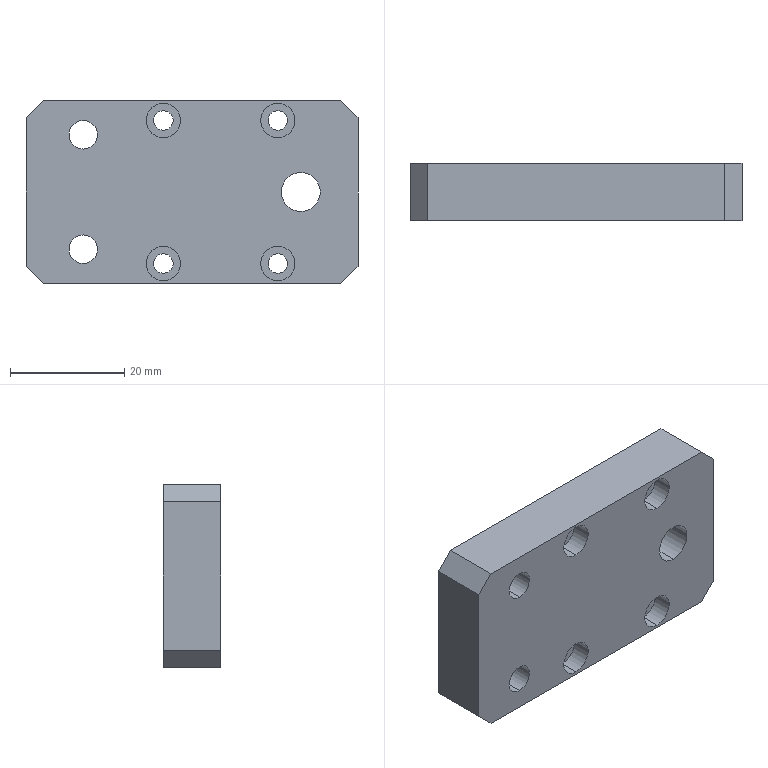Part | SolidWorks | features HoleWzd 3, Chamfer 1, Extrusion 1 | 1 solid | 36 faces | box 58 x 10 x 32 mm | volume 17000 mm3 | cylinder 22 | plane 14 | commonest cylinder face diameters 3.4 x8 6 x8 5 x4 6.8 x2
STEP:
#1=CARTESIAN_POINT('',(19.,10.,-3.4));
#2=VERTEX_POINT('',#1);
#3=CARTESIAN_POINT('',(19.,10.,3.4));
#4=VERTEX_POINT('',#3);
#5=CARTESIAN_POINT('',(19.,10.,0.));
#6=DIRECTION('',(0.,1.,0.));
#7=DIRECTION('',(0.,0.,1.));
#8=AXIS2_PLACEMENT_3D('',#5,#6,#7);
#9=CIRCLE('',#8,3.4);
#10=EDGE_CURVE('',#2,#4,#9,.T.);
#11=ORIENTED_EDGE('',*,*,#10,.T.);
#12=CARTESIAN_POINT('',(19.,0.,3.4));
#13=VERTEX_POINT('',#12);
#14=CARTESIAN_POINT('',(19.,0.,3.4));
#15=DIRECTION('',(0.,-1.,0.));
#16=VECTOR('',#15,1000.);
#17=LINE('',#14,#16);
#18=EDGE_CURVE('',#4,#13,#17,.T.);
#19=ORIENTED_EDGE('',*,*,#18,.T.);
#20=CARTESIAN_POINT('',(19.,0.,-3.4));
#21=VERTEX_POINT('',#20);
#22=CARTESIAN_POINT('',(19.,0.,0.));
#23=DIRECTION('',(0.,-1.,0.));
#24=DIRECTION('',(0.,0.,-1.));
#25=AXIS2_PLACEMENT_3D('',#22,#23,#24);
#26=CIRCLE('',#25,3.4);
#27=EDGE_CURVE('',#13,#21,#26,.T.);
#28=ORIENTED_EDGE('',*,*,#27,.T.);
#29=CARTESIAN_POINT('',(19.,0.,-3.4));
#30=DIRECTION('',(0.,-1.,0.));
#31=VECTOR('',#30,1000.);
#32=LINE('',#29,#31);
#33=EDGE_CURVE('',#2,#21,#32,.T.);
#34=ORIENTED_EDGE('',*,*,#33,.F.);
#35=EDGE_LOOP('',(#11,#19,#28,#34));
#36=FACE_OUTER_BOUND('',#35,.T.);
#37=CARTESIAN_POINT('',(19.,0.,0.));
#38=DIRECTION('',(0.,-1.,0.));
#39=DIRECTION('',(0.,0.,-1.));
#40=AXIS2_PLACEMENT_3D('',#37,#38,#39);
#41=CYLINDRICAL_SURFACE('',#40,3.4);
#42=ADVANCED_FACE('',(#36),#41,.F.);
#43=CARTESIAN_POINT('',(-19.,10.,-12.5));
#44=VERTEX_POINT('',#43);
#45=CARTESIAN_POINT('',(-19.,10.,-7.5));
#46=VERTEX_POINT('',#45);
#47=CARTESIAN_POINT('',(-19.,10.,-10.));
#48=DIRECTION('',(0.,1.,0.));
#49=DIRECTION('',(0.,0.,1.));
#50=AXIS2_PLACEMENT_3D('',#47,#48,#49);
#51=CIRCLE('',#50,2.5);
#52=EDGE_CURVE('',#44,#46,#51,.T.);
#53=ORIENTED_EDGE('',*,*,#52,.T.);
#54=CARTESIAN_POINT('',(-19.,0.,-7.5));
#55=VERTEX_POINT('',#54);
#56=CARTESIAN_POINT('',(-19.,0.,-7.5));
#57=DIRECTION('',(0.,-1.,0.));
#58=VECTOR('',#57,1000.);
#59=LINE('',#56,#58);
#60=EDGE_CURVE('',#46,#55,#59,.T.);
#61=ORIENTED_EDGE('',*,*,#60,.T.);
#62=CARTESIAN_POINT('',(-19.,0.,-12.5));
#63=VERTEX_POINT('',#62);
#64=CARTESIAN_POINT('',(-19.,0.,-10.));
#65=DIRECTION('',(0.,-1.,0.));
#66=DIRECTION('',(0.,0.,-1.));
#67=AXIS2_PLACEMENT_3D('',#64,#65,#66);
#68=CIRCLE('',#67,2.5);
#69=EDGE_CURVE('',#55,#63,#68,.T.);
#70=ORIENTED_EDGE('',*,*,#69,.T.);
#71=CARTESIAN_POINT('',(-19.,0.,-12.5));
#72=DIRECTION('',(0.,-1.,0.));
#73=VECTOR('',#72,1000.);
#74=LINE('',#71,#73);
#75=EDGE_CURVE('',#44,#63,#74,.T.);
#76=ORIENTED_EDGE('',*,*,#75,.F.);
#77=EDGE_LOOP('',(#53,#61,#70,#76));
#78=FACE_OUTER_BOUND('',#77,.T.);
#79=CARTESIAN_POINT('',(-19.,0.,-10.));
#80=DIRECTION('',(0.,-1.,0.));
#81=DIRECTION('',(0.,0.,-1.));
#82=AXIS2_PLACEMENT_3D('',#79,#80,#81);
#83=CYLINDRICAL_SURFACE('',#82,2.5);
#84=ADVANCED_FACE('',(#78),#83,.F.);
#85=CARTESIAN_POINT('',(-19.,10.,7.5));
#86=VERTEX_POINT('',#85);
#87=CARTESIAN_POINT('',(-19.,10.,12.5));
#88=VERTEX_POINT('',#87);
#89=CARTESIAN_POINT('',(-19.,10.,10.));
#90=DIRECTION('',(0.,1.,0.));
#91=DIRECTION('',(0.,0.,1.));
#92=AXIS2_PLACEMENT_3D('',#89,#90,#91);
#93=CIRCLE('',#92,2.5);
#94=EDGE_CURVE('',#86,#88,#93,.T.);
#95=ORIENTED_EDGE('',*,*,#94,.T.);
#96=CARTESIAN_POINT('',(-19.,0.,12.5));
#97=VERTEX_POINT('',#96);
#98=CARTESIAN_POINT('',(-19.,0.,12.5));
#99=DIRECTION('',(0.,-1.,0.));
#100=VECTOR('',#99,1000.);
#101=LINE('',#98,#100);
#102=EDGE_CURVE('',#88,#97,#101,.T.);
#103=ORIENTED_EDGE('',*,*,#102,.T.);
#104=CARTESIAN_POINT('',(-19.,0.,7.5));
#105=VERTEX_POINT('',#104);
#106=CARTESIAN_POINT('',(-19.,0.,10.));
#107=DIRECTION('',(0.,-1.,0.));
#108=DIRECTION('',(0.,0.,-1.));
#109=AXIS2_PLACEMENT_3D('',#106,#107,#108);
#110=CIRCLE('',#109,2.5);
#111=EDGE_CURVE('',#97,#105,#110,.T.);
#112=ORIENTED_EDGE('',*,*,#111,.T.);
#113=CARTESIAN_POINT('',(-19.,0.,7.5));
#114=DIRECTION('',(0.,-1.,0.));
#115=VECTOR('',#114,1000.);
#116=LINE('',#113,#115);
#117=EDGE_CURVE('',#86,#105,#116,.T.);
#118=ORIENTED_EDGE('',*,*,#117,.F.);
#119=EDGE_LOOP('',(#95,#103,#112,#118));
#120=FACE_OUTER_BOUND('',#119,.T.);
#121=CARTESIAN_POINT('',(-19.,0.,10.));
#122=DIRECTION('',(0.,-1.,0.));
#123=DIRECTION('',(0.,0.,-1.));
#124=AXIS2_PLACEMENT_3D('',#121,#122,#123);
#125=CYLINDRICAL_SURFACE('',#124,2.5);
#126=ADVANCED_FACE('',(#120),#125,.F.);
#127=CARTESIAN_POINT('',(15.,3.4,-9.5));
#128=VERTEX_POINT('',#127);
#129=CARTESIAN_POINT('',(15.,3.4,-15.5));
#130=VERTEX_POINT('',#129);
#131=CARTESIAN_POINT('',(15.,3.4,-12.5));
#132=DIRECTION('',(0.,-1.,0.));
#133=DIRECTION('',(0.,0.,-1.));
#134=AXIS2_PLACEMENT_3D('',#131,#132,#133);
#135=CIRCLE('',#134,3.);
#136=EDGE_CURVE('',#128,#130,#135,.T.);
#137=ORIENTED_EDGE('',*,*,#136,.F.);
#138=CARTESIAN_POINT('',(15.,0.,-9.5));
#139=VERTEX_POINT('',#138);
#140=CARTESIAN_POINT('',(15.,0.,-9.5));
#141=DIRECTION('',(0.,-1.,0.));
#142=VECTOR('',#141,1000.);
#143=LINE('',#140,#142);
#144=EDGE_CURVE('',#128,#139,#143,.T.);
#145=ORIENTED_EDGE('',*,*,#144,.T.);
#146=CARTESIAN_POINT('',(15.,0.,-15.5));
#147=VERTEX_POINT('',#146);
#148=CARTESIAN_POINT('',(15.,0.,-12.5));
#149=DIRECTION('',(0.,-1.,0.));
#150=DIRECTION('',(0.,0.,-1.));
#151=AXIS2_PLACEMENT_3D('',#148,#149,#150);
#152=CIRCLE('',#151,3.);
#153=EDGE_CURVE('',#139,#147,#152,.T.);
#154=ORIENTED_EDGE('',*,*,#153,.T.);
#155=CARTESIAN_POINT('',(15.,0.,-15.5));
#156=DIRECTION('',(0.,-1.,0.));
#157=VECTOR('',#156,1000.);
#158=LINE('',#155,#157);
#159=EDGE_CURVE('',#130,#147,#158,.T.);
#160=ORIENTED_EDGE('',*,*,#159,.F.);
#161=EDGE_LOOP('',(#137,#145,#154,#160));
#162=FACE_OUTER_BOUND('',#161,.T.);
#163=CARTESIAN_POINT('',(15.,0.,-12.5));
#164=DIRECTION('',(0.,-1.,0.));
#165=DIRECTION('',(0.,0.,-1.));
#166=AXIS2_PLACEMENT_3D('',#163,#164,#165);
#167=CYLINDRICAL_SURFACE('',#166,3.);
#168=ADVANCED_FACE('',(#162),#167,.F.);
#169=CARTESIAN_POINT('',(15.,10.,-14.2));
#170=VERTEX_POINT('',#169);
#171=CARTESIAN_POINT('',(15.,10.,-10.8));
#172=VERTEX_POINT('',#171);
#173=CARTESIAN_POINT('',(15.,10.,-12.5));
#174=DIRECTION('',(0.,1.,0.));
#175=DIRECTION('',(0.,0.,1.));
#176=AXIS2_PLACEMENT_3D('',#173,#174,#175);
#177=CIRCLE('',#176,1.7);
#178=EDGE_CURVE('',#170,#172,#177,.T.);
#179=ORIENTED_EDGE('',*,*,#178,.T.);
#180=CARTESIAN_POINT('',(15.,3.4,-10.8));
#181=VERTEX_POINT('',#180);
#182=CARTESIAN_POINT('',(15.,0.,-10.8));
#183=DIRECTION('',(0.,-1.,0.));
#184=VECTOR('',#183,1000.);
#185=LINE('',#182,#184);
#186=EDGE_CURVE('',#172,#181,#185,.T.);
#187=ORIENTED_EDGE('',*,*,#186,.T.);
#188=CARTESIAN_POINT('',(15.,3.4,-14.2));
#189=VERTEX_POINT('',#188);
#190=CARTESIAN_POINT('',(15.,3.4,-12.5));
#191=DIRECTION('',(0.,-1.,0.));
#192=DIRECTION('',(0.,0.,-1.));
#193=AXIS2_PLACEMENT_3D('',#190,#191,#192);
#194=CIRCLE('',#193,1.7);
#195=EDGE_CURVE('',#181,#189,#194,.T.);
#196=ORIENTED_EDGE('',*,*,#195,.T.);
#197=CARTESIAN_POINT('',(15.,0.,-14.2));
#198=DIRECTION('',(0.,-1.,0.));
#199=VECTOR('',#198,1000.);
#200=LINE('',#197,#199);
#201=EDGE_CURVE('',#170,#189,#200,.T.);
#202=ORIENTED_EDGE('',*,*,#201,.F.);
#203=EDGE_LOOP('',(#179,#187,#196,#202));
#204=FACE_OUTER_BOUND('',#203,.T.);
#205=CARTESIAN_POINT('',(15.,0.,-12.5));
#206=DIRECTION('',(0.,-1.,0.));
#207=DIRECTION('',(0.,0.,-1.));
#208=AXIS2_PLACEMENT_3D('',#205,#206,#207);
#209=CYLINDRICAL_SURFACE('',#208,1.7);
#210=ADVANCED_FACE('',(#204),#209,.F.);
#211=CARTESIAN_POINT('',(-5.,3.4,-9.5));
#212=VERTEX_POINT('',#211);
#213=CARTESIAN_POINT('',(-5.,3.4,-15.5));
#214=VERTEX_POINT('',#213);
#215=CARTESIAN_POINT('',(-5.,3.4,-12.5));
#216=DIRECTION('',(0.,-1.,0.));
#217=DIRECTION('',(0.,0.,-1.));
#218=AXIS2_PLACEMENT_3D('',#215,#216,#217);
#219=CIRCLE('',#218,3.);
#220=EDGE_CURVE('',#212,#214,#219,.T.);
#221=ORIENTED_EDGE('',*,*,#220,.F.);
#222=CARTESIAN_POINT('',(-5.,0.,-9.5));
#223=VERTEX_POINT('',#222);
#224=CARTESIAN_POINT('',(-5.,0.,-9.5));
#225=DIRECTION('',(0.,-1.,0.));
#226=VECTOR('',#225,1000.);
#227=LINE('',#224,#226);
#228=EDGE_CURVE('',#212,#223,#227,.T.);
#229=ORIENTED_EDGE('',*,*,#228,.T.);
#230=CARTESIAN_POINT('',(-5.,0.,-15.5));
#231=VERTEX_POINT('',#230);
#232=CARTESIAN_POINT('',(-5.,0.,-12.5));
#233=DIRECTION('',(0.,-1.,0.));
#234=DIRECTION('',(0.,0.,-1.));
#235=AXIS2_PLACEMENT_3D('',#232,#233,#234);
#236=CIRCLE('',#235,3.);
#237=EDGE_CURVE('',#223,#231,#236,.T.);
#238=ORIENTED_EDGE('',*,*,#237,.T.);
#239=CARTESIAN_POINT('',(-5.,0.,-15.5));
#240=DIRECTION('',(0.,-1.,0.));
#241=VECTOR('',#240,1000.);
#242=LINE('',#239,#241);
#243=EDGE_CURVE('',#214,#231,#242,.T.);
#244=ORIENTED_EDGE('',*,*,#243,.F.);
#245=EDGE_LOOP('',(#221,#229,#238,#244));
#246=FACE_OUTER_BOUND('',#245,.T.);
#247=CARTESIAN_POINT('',(-5.,0.,-12.5));
#248=DIRECTION('',(0.,-1.,0.));
#249=DIRECTION('',(0.,0.,-1.));
#250=AXIS2_PLACEMENT_3D('',#247,#248,#249);
#251=CYLINDRICAL_SURFACE('',#250,3.);
#252=ADVANCED_FACE('',(#246),#251,.F.);
#253=CARTESIAN_POINT('',(-5.,10.,-14.2));
#254=VERTEX_POINT('',#253);
#255=CARTESIAN_POINT('',(-5.,10.,-10.8));
#256=VERTEX_POINT('',#255);
#257=CARTESIAN_POINT('',(-5.,10.,-12.5));
#258=DIRECTION('',(0.,1.,0.));
#259=DIRECTION('',(0.,0.,1.));
#260=AXIS2_PLACEMENT_3D('',#257,#258,#259);
#261=CIRCLE('',#260,1.7);
#262=EDGE_CURVE('',#254,#256,#261,.T.);
#263=ORIENTED_EDGE('',*,*,#262,.T.);
#264=CARTESIAN_POINT('',(-5.,3.4,-10.8));
#265=VERTEX_POINT('',#264);
#266=CARTESIAN_POINT('',(-5.,0.,-10.8));
#267=DIRECTION('',(0.,-1.,0.));
#268=VECTOR('',#267,1000.);
#269=LINE('',#266,#268);
#270=EDGE_CURVE('',#256,#265,#269,.T.);
#271=ORIENTED_EDGE('',*,*,#270,.T.);
#272=CARTESIAN_POINT('',(-5.,3.4,-14.2));
#273=VERTEX_POINT('',#272);
#274=CARTESIAN_POINT('',(-5.,3.4,-12.5));
#275=DIRECTION('',(0.,-1.,0.));
#276=DIRECTION('',(0.,0.,-1.));
#277=AXIS2_PLACEMENT_3D('',#274,#275,#276);
#278=CIRCLE('',#277,1.7);
#279=EDGE_CURVE('',#265,#273,#278,.T.);
#280=ORIENTED_EDGE('',*,*,#279,.T.);
#281=CARTESIAN_POINT('',(-5.,0.,-14.2));
#282=DIRECTION('',(0.,-1.,0.));
#283=VECTOR('',#282,1000.);
#284=LINE('',#281,#283);
#285=EDGE_CURVE('',#254,#273,#284,.T.);
#286=ORIENTED_EDGE('',*,*,#285,.F.);
#287=EDGE_LOOP('',(#263,#271,#280,#286));
#288=FACE_OUTER_BOUND('',#287,.T.);
#289=CARTESIAN_POINT('',(-5.,0.,-12.5));
#290=DIRECTION('',(0.,-1.,0.));
#291=DIRECTION('',(0.,0.,-1.));
#292=AXIS2_PLACEMENT_3D('',#289,#290,#291);
#293=CYLINDRICAL_SURFACE('',#292,1.7);
#294=ADVANCED_FACE('',(#288),#293,.F.);
#295=CARTESIAN_POINT('',(15.,3.4,15.5));
#296=VERTEX_POINT('',#295);
#297=CARTESIAN_POINT('',(15.,3.4,9.5));
#298=VERTEX_POINT('',#297);
#299=CARTESIAN_POINT('',(15.,3.4,12.5));
#300=DIRECTION('',(0.,-1.,0.));
#301=DIRECTION('',(0.,0.,-1.));
#302=AXIS2_PLACEMENT_3D('',#299,#300,#301);
#303=CIRCLE('',#302,3.);
#304=EDGE_CURVE('',#296,#298,#303,.T.);
#305=ORIENTED_EDGE('',*,*,#304,.F.);
#306=CARTESIAN_POINT('',(15.,0.,15.5));
#307=VERTEX_POINT('',#306);
#308=CARTESIAN_POINT('',(15.,0.,15.5));
#309=DIRECTION('',(0.,-1.,0.));
#310=VECTOR('',#309,1000.);
#311=LINE('',#308,#310);
#312=EDGE_CURVE('',#296,#307,#311,.T.);
#313=ORIENTED_EDGE('',*,*,#312,.T.);
#314=CARTESIAN_POINT('',(15.,0.,9.5));
#315=VERTEX_POINT('',#314);
#316=CARTESIAN_POINT('',(15.,0.,12.5));
#317=DIRECTION('',(0.,-1.,0.));
#318=DIRECTION('',(0.,0.,-1.));
#319=AXIS2_PLACEMENT_3D('',#316,#317,#318);
#320=CIRCLE('',#319,3.);
#321=EDGE_CURVE('',#307,#315,#320,.T.);
#322=ORIENTED_EDGE('',*,*,#321,.T.);
#323=CARTESIAN_POINT('',(15.,0.,9.5));
#324=DIRECTION('',(0.,-1.,0.));
#325=VECTOR('',#324,1000.);
#326=LINE('',#323,#325);
#327=EDGE_CURVE('',#298,#315,#326,.T.);
#328=ORIENTED_EDGE('',*,*,#327,.F.);
#329=EDGE_LOOP('',(#305,#313,#322,#328));
#330=FACE_OUTER_BOUND('',#329,.T.);
#331=CARTESIAN_POINT('',(15.,0.,12.5));
#332=DIRECTION('',(0.,-1.,0.));
#333=DIRECTION('',(0.,0.,-1.));
#334=AXIS2_PLACEMENT_3D('',#331,#332,#333);
#335=CYLINDRICAL_SURFACE('',#334,3.);
#336=ADVANCED_FACE('',(#330),#335,.F.);
#337=CARTESIAN_POINT('',(15.,10.,10.8));
#338=VERTEX_POINT('',#337);
#339=CARTESIAN_POINT('',(15.,10.,14.2));
#340=VERTEX_POINT('',#339);
#341=CARTESIAN_POINT('',(15.,10.,12.5));
#342=DIRECTION('',(0.,1.,0.));
#343=DIRECTION('',(0.,0.,1.));
#344=AXIS2_PLACEMENT_3D('',#341,#342,#343);
#345=CIRCLE('',#344,1.7);
#346=EDGE_CURVE('',#338,#340,#345,.T.);
#347=ORIENTED_EDGE('',*,*,#346,.T.);
#348=CARTESIAN_POINT('',(15.,3.4,14.2));
#349=VERTEX_POINT('',#348);
#350=CARTESIAN_POINT('',(15.,0.,14.2));
#351=DIRECTION('',(0.,-1.,0.));
#352=VECTOR('',#351,1000.);
#353=LINE('',#350,#352);
#354=EDGE_CURVE('',#340,#349,#353,.T.);
#355=ORIENTED_EDGE('',*,*,#354,.T.);
#356=CARTESIAN_POINT('',(15.,3.4,10.8));
#357=VERTEX_POINT('',#356);
#358=CARTESIAN_POINT('',(15.,3.4,12.5));
#359=DIRECTION('',(0.,-1.,0.));
#360=DIRECTION('',(0.,0.,-1.));
#361=AXIS2_PLACEMENT_3D('',#358,#359,#360);
#362=CIRCLE('',#361,1.7);
#363=EDGE_CURVE('',#349,#357,#362,.T.);
#364=ORIENTED_EDGE('',*,*,#363,.T.);
#365=CARTESIAN_POINT('',(15.,0.,10.8));
#366=DIRECTION('',(0.,-1.,0.));
#367=VECTOR('',#366,1000.);
#368=LINE('',#365,#367);
#369=EDGE_CURVE('',#338,#357,#368,.T.);
#370=ORIENTED_EDGE('',*,*,#369,.F.);
#371=EDGE_LOOP('',(#347,#355,#364,#370));
#372=FACE_OUTER_BOUND('',#371,.T.);
#373=CARTESIAN_POINT('',(15.,0.,12.5));
#374=DIRECTION('',(0.,-1.,0.));
#375=DIRECTION('',(0.,0.,-1.));
#376=AXIS2_PLACEMENT_3D('',#373,#374,#375);
#377=CYLINDRICAL_SURFACE('',#376,1.7);
#378=ADVANCED_FACE('',(#372),#377,.F.);
#379=CARTESIAN_POINT('',(-5.,3.4,15.5));
#380=VERTEX_POINT('',#379);
#381=CARTESIAN_POINT('',(-5.,3.4,9.5));
#382=VERTEX_POINT('',#381);
#383=CARTESIAN_POINT('',(-5.,3.4,12.5));
#384=DIRECTION('',(0.,-1.,0.));
#385=DIRECTION('',(0.,0.,-1.));
#386=AXIS2_PLACEMENT_3D('',#383,#384,#385);
#387=CIRCLE('',#386,3.);
#388=EDGE_CURVE('',#380,#382,#387,.T.);
#389=ORIENTED_EDGE('',*,*,#388,.F.);
#390=CARTESIAN_POINT('',(-5.,0.,15.5));
#391=VERTEX_POINT('',#390);
#392=CARTESIAN_POINT('',(-5.,0.,15.5));
#393=DIRECTION('',(0.,-1.,0.));
#394=VECTOR('',#393,1000.);
#395=LINE('',#392,#394);
#396=EDGE_CURVE('',#380,#391,#395,.T.);
#397=ORIENTED_EDGE('',*,*,#396,.T.);
#398=CARTESIAN_POINT('',(-5.,0.,9.5));
#399=VERTEX_POINT('',#398);
#400=CARTESIAN_POINT('',(-5.,0.,12.5));
#401=DIRECTION('',(0.,-1.,0.));
#402=DIRECTION('',(0.,0.,-1.));
#403=AXIS2_PLACEMENT_3D('',#400,#401,#402);
#404=CIRCLE('',#403,3.);
#405=EDGE_CURVE('',#391,#399,#404,.T.);
#406=ORIENTED_EDGE('',*,*,#405,.T.);
#407=CARTESIAN_POINT('',(-5.,0.,9.5));
#408=DIRECTION('',(0.,-1.,0.));
#409=VECTOR('',#408,1000.);
#410=LINE('',#407,#409);
#411=EDGE_CURVE('',#382,#399,#410,.T.);
#412=ORIENTED_EDGE('',*,*,#411,.F.);
#413=EDGE_LOOP('',(#389,#397,#406,#412));
#414=FACE_OUTER_BOUND('',#413,.T.);
#415=CARTESIAN_POINT('',(-5.,0.,12.5));
#416=DIRECTION('',(0.,-1.,0.));
#417=DIRECTION('',(0.,0.,-1.));
#418=AXIS2_PLACEMENT_3D('',#415,#416,#417);
#419=CYLINDRICAL_SURFACE('',#418,3.);
#420=ADVANCED_FACE('',(#414),#419,.F.);
#421=CARTESIAN_POINT('',(-5.,10.,10.8));
#422=VERTEX_POINT('',#421);
#423=CARTESIAN_POINT('',(-5.,10.,14.2));
#424=VERTEX_POINT('',#423);
#425=CARTESIAN_POINT('',(-5.,10.,12.5));
#426=DIRECTION('',(0.,1.,0.));
#427=DIRECTION('',(0.,0.,1.));
#428=AXIS2_PLACEMENT_3D('',#425,#426,#427);
#429=CIRCLE('',#428,1.7);
#430=EDGE_CURVE('',#422,#424,#429,.T.);
#431=ORIENTED_EDGE('',*,*,#430,.T.);
#432=CARTESIAN_POINT('',(-5.,3.4,14.2));
#433=VERTEX_POINT('',#432);
#434=CARTESIAN_POINT('',(-5.,0.,14.2));
#435=DIRECTION('',(0.,-1.,0.));
#436=VECTOR('',#435,1000.);
#437=LINE('',#434,#436);
#438=EDGE_CURVE('',#424,#433,#437,.T.);
#439=ORIENTED_EDGE('',*,*,#438,.T.);
#440=CARTESIAN_POINT('',(-5.,3.4,10.8));
#441=VERTEX_POINT('',#440);
#442=CARTESIAN_POINT('',(-5.,3.4,12.5));
#443=DIRECTION('',(0.,-1.,0.));
#444=DIRECTION('',(0.,0.,-1.));
#445=AXIS2_PLACEMENT_3D('',#442,#443,#444);
#446=CIRCLE('',#445,1.7);
#447=EDGE_CURVE('',#433,#441,#446,.T.);
#448=ORIENTED_EDGE('',*,*,#447,.T.);
#449=CARTESIAN_POINT('',(-5.,0.,10.8));
#450=DIRECTION('',(0.,-1.,0.));
#451=VECTOR('',#450,1000.);
#452=LINE('',#449,#451);
#453=EDGE_CURVE('',#422,#441,#452,.T.);
#454=ORIENTED_EDGE('',*,*,#453,.F.);
#455=EDGE_LOOP('',(#431,#439,#448,#454));
#456=FACE_OUTER_BOUND('',#455,.T.);
#457=CARTESIAN_POINT('',(-5.,0.,12.5));
#458=DIRECTION('',(0.,-1.,0.));
#459=DIRECTION('',(0.,0.,-1.));
#460=AXIS2_PLACEMENT_3D('',#457,#458,#459);
#461=CYLINDRICAL_SURFACE('',#460,1.7);
#462=ADVANCED_FACE('',(#456),#461,.F.);
#463=CARTESIAN_POINT('',(29.,0.,13.));
#464=VERTEX_POINT('',#463);
#465=CARTESIAN_POINT('',(29.,0.,-13.));
#466=VERTEX_POINT('',#465);
#467=CARTESIAN_POINT('',(29.,0.,-16.));
#468=DIRECTION('',(0.,0.,-1.));
#469=VECTOR('',#468,1000.);
#470=LINE('',#467,#469);
#471=EDGE_CURVE('',#464,#466,#470,.T.);
#472=ORIENTED_EDGE('',*,*,#471,.T.);
#473=CARTESIAN_POINT('',(29.,10.,-13.));
#474=VERTEX_POINT('',#473);
#475=CARTESIAN_POINT('',(29.,10.,-13.));
#476=DIRECTION('',(0.,1.,0.));
#477=VECTOR('',#476,1000.);
#478=LINE('',#475,#477);
#479=EDGE_CURVE('',#466,#474,#478,.T.);
#480=ORIENTED_EDGE('',*,*,#479,.T.);
#481=CARTESIAN_POINT('',(29.,10.,13.));
#482=VERTEX_POINT('',#481);
#483=CARTESIAN_POINT('',(29.,10.,-16.));
#484=DIRECTION('',(0.,0.,-1.));
#485=VECTOR('',#484,1000.);
#486=LINE('',#483,#485);
#487=EDGE_CURVE('',#482,#474,#486,.T.);
#488=ORIENTED_EDGE('',*,*,#487,.F.);
#489=CARTESIAN_POINT('',(29.,10.,13.));
#490=DIRECTION('',(0.,-1.,0.));
#491=VECTOR('',#490,1000.);
#492=LINE('',#489,#491);
#493=EDGE_CURVE('',#482,#464,#492,.T.);
#494=ORIENTED_EDGE('',*,*,#493,.T.);
#495=EDGE_LOOP('',(#472,#480,#488,#494));
#496=FACE_OUTER_BOUND('',#495,.T.);
#497=CARTESIAN_POINT('',(29.,10.,-16.));
#498=DIRECTION('',(-1.,0.,0.));
#499=DIRECTION('',(0.,0.,1.));
#500=AXIS2_PLACEMENT_3D('',#497,#498,#499);
#501=PLANE('',#500);
#502=ADVANCED_FACE('',(#496),#501,.F.);
#503=CARTESIAN_POINT('',(26.,0.,-16.));
#504=VERTEX_POINT('',#503);
#505=CARTESIAN_POINT('',(-26.,0.,-16.));
#506=VERTEX_POINT('',#505);
#507=CARTESIAN_POINT('',(-29.,0.,-16.));
#508=DIRECTION('',(-1.,0.,0.));
#509=VECTOR('',#508,1000.);
#510=LINE('',#507,#509);
#511=EDGE_CURVE('',#504,#506,#510,.T.);
#512=ORIENTED_EDGE('',*,*,#511,.T.);
#513=CARTESIAN_POINT('',(-26.,10.,-16.));
#514=VERTEX_POINT('',#513);
#515=CARTESIAN_POINT('',(-26.,10.,-16.));
#516=DIRECTION('',(0.,1.,0.));
#517=VECTOR('',#516,1000.);
#518=LINE('',#515,#517);
#519=EDGE_CURVE('',#506,#514,#518,.T.);
#520=ORIENTED_EDGE('',*,*,#519,.T.);
#521=CARTESIAN_POINT('',(26.,10.,-16.));
#522=VERTEX_POINT('',#521);
#523=CARTESIAN_POINT('',(-29.,10.,-16.));
#524=DIRECTION('',(-1.,0.,0.));
#525=VECTOR('',#524,1000.);
#526=LINE('',#523,#525);
#527=EDGE_CURVE('',#522,#514,#526,.T.);
#528=ORIENTED_EDGE('',*,*,#527,.F.);
#529=CARTESIAN_POINT('',(26.,10.,-16.));
#530=DIRECTION('',(0.,-1.,0.));
#531=VECTOR('',#530,1000.);
#532=LINE('',#529,#531);
#533=EDGE_CURVE('',#522,#504,#532,.T.);
#534=ORIENTED_EDGE('',*,*,#533,.T.);
#535=EDGE_LOOP('',(#512,#520,#528,#534));
#536=FACE_OUTER_BOUND('',#535,.T.);
#537=CARTESIAN_POINT('',(-29.,10.,-16.));
#538=DIRECTION('',(0.,0.,1.));
#539=DIRECTION('',(1.,0.,0.));
#540=AXIS2_PLACEMENT_3D('',#537,#538,#539);
#541=PLANE('',#540);
#542=ADVANCED_FACE('',(#536),#541,.F.);
#543=CARTESIAN_POINT('',(-29.,10.,-13.));
#544=VERTEX_POINT('',#543);
#545=CARTESIAN_POINT('',(-29.,10.,13.));
#546=VERTEX_POINT('',#545);
#547=CARTESIAN_POINT('',(-29.,10.,-16.));
#548=DIRECTION('',(0.,0.,1.));
#549=VECTOR('',#548,1000.);
#550=LINE('',#547,#549);
#551=EDGE_CURVE('',#544,#546,#550,.T.);
#552=ORIENTED_EDGE('',*,*,#551,.F.);
#553=CARTESIAN_POINT('',(-29.,0.,-13.));
#554=VERTEX_POINT('',#553);
#555=CARTESIAN_POINT('',(-29.,10.,-13.));
#556=DIRECTION('',(0.,-1.,0.));
#557=VECTOR('',#556,1000.);
#558=LINE('',#555,#557);
#559=EDGE_CURVE('',#544,#554,#558,.T.);
#560=ORIENTED_EDGE('',*,*,#559,.T.);
#561=CARTESIAN_POINT('',(-29.,0.,13.));
#562=VERTEX_POINT('',#561);
#563=CARTESIAN_POINT('',(-29.,0.,-16.));
#564=DIRECTION('',(0.,0.,1.));
#565=VECTOR('',#564,1000.);
#566=LINE('',#563,#565);
#567=EDGE_CURVE('',#554,#562,#566,.T.);
#568=ORIENTED_EDGE('',*,*,#567,.T.);
#569=CARTESIAN_POINT('',(-29.,10.,13.));
#570=DIRECTION('',(0.,1.,0.));
#571=VECTOR('',#570,1000.);
#572=LINE('',#569,#571);
#573=EDGE_CURVE('',#562,#546,#572,.T.);
#574=ORIENTED_EDGE('',*,*,#573,.T.);
#575=EDGE_LOOP('',(#552,#560,#568,#574));
#576=FACE_OUTER_BOUND('',#575,.T.);
#577=CARTESIAN_POINT('',(-29.,10.,-16.));
#578=DIRECTION('',(1.,0.,0.));
#579=DIRECTION('',(0.,0.,-1.));
#580=AXIS2_PLACEMENT_3D('',#577,#578,#579);
#581=PLANE('',#580);
#582=ADVANCED_FACE('',(#576),#581,.F.);
#583=CARTESIAN_POINT('',(-26.,10.,16.));
#584=VERTEX_POINT('',#583);
#585=CARTESIAN_POINT('',(26.,10.,16.));
#586=VERTEX_POINT('',#585);
#587=CARTESIAN_POINT('',(-29.,10.,16.));
#588=DIRECTION('',(1.,0.,0.));
#589=VECTOR('',#588,1000.);
#590=LINE('',#587,#589);
#591=EDGE_CURVE('',#584,#586,#590,.T.);
#592=ORIENTED_EDGE('',*,*,#591,.F.);
#593=CARTESIAN_POINT('',(-26.,0.,16.));
#594=VERTEX_POINT('',#593);
#595=CARTESIAN_POINT('',(-26.,10.,16.));
#596=DIRECTION('',(0.,-1.,0.));
#597=VECTOR('',#596,1000.);
#598=LINE('',#595,#597);
#599=EDGE_CURVE('',#584,#594,#598,.T.);
#600=ORIENTED_EDGE('',*,*,#599,.T.);
#601=CARTESIAN_POINT('',(26.,0.,16.));
#602=VERTEX_POINT('',#601);
#603=CARTESIAN_POINT('',(-29.,0.,16.));
#604=DIRECTION('',(1.,0.,0.));
#605=VECTOR('',#604,1000.);
#606=LINE('',#603,#605);
#607=EDGE_CURVE('',#594,#602,#606,.T.);
#608=ORIENTED_EDGE('',*,*,#607,.T.);
#609=CARTESIAN_POINT('',(26.,10.,16.));
#610=DIRECTION('',(0.,1.,0.));
#611=VECTOR('',#610,1000.);
#612=LINE('',#609,#611);
#613=EDGE_CURVE('',#602,#586,#612,.T.);
#614=ORIENTED_EDGE('',*,*,#613,.T.);
#615=EDGE_LOOP('',(#592,#600,#608,#614));
#616=FACE_OUTER_BOUND('',#615,.T.);
#617=CARTESIAN_POINT('',(-29.,10.,16.));
#618=DIRECTION('',(0.,0.,-1.));
#619=DIRECTION('',(-1.,0.,0.));
#620=AXIS2_PLACEMENT_3D('',#617,#618,#619);
#621=PLANE('',#620);
#622=ADVANCED_FACE('',(#616),#621,.F.);
#623=ORIENTED_EDGE('',*,*,#10,.F.);
#624=CARTESIAN_POINT('',(19.,10.,0.));
#625=DIRECTION('',(0.,1.,0.));
#626=DIRECTION('',(0.,0.,1.));
#627=AXIS2_PLACEMENT_3D('',#624,#625,#626);
#628=CIRCLE('',#627,3.4);
#629=EDGE_CURVE('',#4,#2,#628,.T.);
#630=ORIENTED_EDGE('',*,*,#629,.F.);
#631=EDGE_LOOP('',(#623,#630));
#632=FACE_BOUND('',#631,.T.);
#633=ORIENTED_EDGE('',*,*,#52,.F.);
#634=CARTESIAN_POINT('',(-19.,10.,-10.));
#635=DIRECTION('',(0.,1.,0.));
#636=DIRECTION('',(0.,0.,1.));
#637=AXIS2_PLACEMENT_3D('',#634,#635,#636);
#638=CIRCLE('',#637,2.5);
#639=EDGE_CURVE('',#46,#44,#638,.T.);
#640=ORIENTED_EDGE('',*,*,#639,.F.);
#641=EDGE_LOOP('',(#633,#640));
#642=FACE_BOUND('',#641,.T.);
#643=ORIENTED_EDGE('',*,*,#94,.F.);
#644=CARTESIAN_POINT('',(-19.,10.,10.));
#645=DIRECTION('',(0.,1.,0.));
#646=DIRECTION('',(0.,0.,1.));
#647=AXIS2_PLACEMENT_3D('',#644,#645,#646);
#648=CIRCLE('',#647,2.5);
#649=EDGE_CURVE('',#88,#86,#648,.T.);
#650=ORIENTED_EDGE('',*,*,#649,.F.);
#651=EDGE_LOOP('',(#643,#650));
#652=FACE_BOUND('',#651,.T.);
#653=ORIENTED_EDGE('',*,*,#178,.F.);
#654=CARTESIAN_POINT('',(15.,10.,-12.5));
#655=DIRECTION('',(0.,1.,0.));
#656=DIRECTION('',(0.,0.,1.));
#657=AXIS2_PLACEMENT_3D('',#654,#655,#656);
#658=CIRCLE('',#657,1.7);
#659=EDGE_CURVE('',#172,#170,#658,.T.);
#660=ORIENTED_EDGE('',*,*,#659,.F.);
#661=EDGE_LOOP('',(#653,#660));
#662=FACE_BOUND('',#661,.T.);
#663=ORIENTED_EDGE('',*,*,#262,.F.);
#664=CARTESIAN_POINT('',(-5.,10.,-12.5));
#665=DIRECTION('',(0.,1.,0.));
#666=DIRECTION('',(0.,0.,1.));
#667=AXIS2_PLACEMENT_3D('',#664,#665,#666);
#668=CIRCLE('',#667,1.7);
#669=EDGE_CURVE('',#256,#254,#668,.T.);
#670=ORIENTED_EDGE('',*,*,#669,.F.);
#671=EDGE_LOOP('',(#663,#670));
#672=FACE_BOUND('',#671,.T.);
#673=ORIENTED_EDGE('',*,*,#346,.F.);
#674=CARTESIAN_POINT('',(15.,10.,12.5));
#675=DIRECTION('',(0.,1.,0.));
#676=DIRECTION('',(0.,0.,1.));
#677=AXIS2_PLACEMENT_3D('',#674,#675,#676);
#678=CIRCLE('',#677,1.7);
#679=EDGE_CURVE('',#340,#338,#678,.T.);
#680=ORIENTED_EDGE('',*,*,#679,.F.);
#681=EDGE_LOOP('',(#673,#680));
#682=FACE_BOUND('',#681,.T.);
#683=ORIENTED_EDGE('',*,*,#430,.F.);
#684=CARTESIAN_POINT('',(-5.,10.,12.5));
#685=DIRECTION('',(0.,1.,0.));
#686=DIRECTION('',(0.,0.,1.));
#687=AXIS2_PLACEMENT_3D('',#684,#685,#686);
#688=CIRCLE('',#687,1.7);
#689=EDGE_CURVE('',#424,#422,#688,.T.);
#690=ORIENTED_EDGE('',*,*,#689,.F.);
#691=EDGE_LOOP('',(#683,#690));
#692=FACE_BOUND('',#691,.T.);
#693=ORIENTED_EDGE('',*,*,#527,.T.);
#694=CARTESIAN_POINT('',(-21.,10.,-21.));
#695=DIRECTION('',(-0.7071,0.,0.7071));
#696=VECTOR('',#695,1000.);
#697=LINE('',#694,#696);
#698=EDGE_CURVE('',#514,#544,#697,.T.);
#699=ORIENTED_EDGE('',*,*,#698,.T.);
#700=ORIENTED_EDGE('',*,*,#551,.T.);
#701=CARTESIAN_POINT('',(-21.,10.,21.));
#702=DIRECTION('',(0.7071,0.,0.7071));
#703=VECTOR('',#702,1000.);
#704=LINE('',#701,#703);
#705=EDGE_CURVE('',#546,#584,#704,.T.);
#706=ORIENTED_EDGE('',*,*,#705,.T.);
#707=ORIENTED_EDGE('',*,*,#591,.T.);
#708=CARTESIAN_POINT('',(21.,10.,21.));
#709=DIRECTION('',(0.7071,0.,-0.7071));
#710=VECTOR('',#709,1000.);
#711=LINE('',#708,#710);
#712=EDGE_CURVE('',#586,#482,#711,.T.);
#713=ORIENTED_EDGE('',*,*,#712,.T.);
#714=ORIENTED_EDGE('',*,*,#487,.T.);
#715=CARTESIAN_POINT('',(21.,10.,-21.));
#716=DIRECTION('',(-0.7071,0.,-0.7071));
#717=VECTOR('',#716,1000.);
#718=LINE('',#715,#717);
#719=EDGE_CURVE('',#474,#522,#718,.T.);
#720=ORIENTED_EDGE('',*,*,#719,.T.);
#721=EDGE_LOOP('',(#693,#699,#700,#706,#707,#713,#714,#720));
#722=FACE_OUTER_BOUND('',#721,.T.);
#723=CARTESIAN_POINT('',(0.,10.,0.));
#724=DIRECTION('',(0.,1.,0.));
#725=DIRECTION('',(0.,0.,1.));
#726=AXIS2_PLACEMENT_3D('',#723,#724,#725);
#727=PLANE('',#726);
#728=ADVANCED_FACE('',(#632,#642,#652,#662,#672,#682,#692,#722),#727,.T.);
#729=CARTESIAN_POINT('',(19.,0.,0.));
#730=DIRECTION('',(0.,-1.,0.));
#731=DIRECTION('',(0.,0.,-1.));
#732=AXIS2_PLACEMENT_3D('',#729,#730,#731);
#733=CIRCLE('',#732,3.4);
#734=EDGE_CURVE('',#21,#13,#733,.T.);
#735=ORIENTED_EDGE('',*,*,#734,.F.);
#736=ORIENTED_EDGE('',*,*,#27,.F.);
#737=EDGE_LOOP('',(#735,#736));
#738=FACE_BOUND('',#737,.T.);
#739=CARTESIAN_POINT('',(-19.,0.,-10.));
#740=DIRECTION('',(0.,-1.,0.));
#741=DIRECTION('',(0.,0.,-1.));
#742=AXIS2_PLACEMENT_3D('',#739,#740,#741);
#743=CIRCLE('',#742,2.5);
#744=EDGE_CURVE('',#63,#55,#743,.T.);
#745=ORIENTED_EDGE('',*,*,#744,.F.);
#746=ORIENTED_EDGE('',*,*,#69,.F.);
#747=EDGE_LOOP('',(#745,#746));
#748=FACE_BOUND('',#747,.T.);
#749=CARTESIAN_POINT('',(-19.,0.,10.));
#750=DIRECTION('',(0.,-1.,0.));
#751=DIRECTION('',(0.,0.,-1.));
#752=AXIS2_PLACEMENT_3D('',#749,#750,#751);
#753=CIRCLE('',#752,2.5);
#754=EDGE_CURVE('',#105,#97,#753,.T.);
#755=ORIENTED_EDGE('',*,*,#754,.F.);
#756=ORIENTED_EDGE('',*,*,#111,.F.);
#757=EDGE_LOOP('',(#755,#756));
#758=FACE_BOUND('',#757,.T.);
#759=CARTESIAN_POINT('',(15.,0.,-12.5));
#760=DIRECTION('',(0.,-1.,0.));
#761=DIRECTION('',(0.,0.,-1.));
#762=AXIS2_PLACEMENT_3D('',#759,#760,#761);
#763=CIRCLE('',#762,3.);
#764=EDGE_CURVE('',#147,#139,#763,.T.);
#765=ORIENTED_EDGE('',*,*,#764,.F.);
#766=ORIENTED_EDGE('',*,*,#153,.F.);
#767=EDGE_LOOP('',(#765,#766));
#768=FACE_BOUND('',#767,.T.);
#769=CARTESIAN_POINT('',(-5.,0.,-12.5));
#770=DIRECTION('',(0.,-1.,0.));
#771=DIRECTION('',(0.,0.,-1.));
#772=AXIS2_PLACEMENT_3D('',#769,#770,#771);
#773=CIRCLE('',#772,3.);
#774=EDGE_CURVE('',#231,#223,#773,.T.);
#775=ORIENTED_EDGE('',*,*,#774,.F.);
#776=ORIENTED_EDGE('',*,*,#237,.F.);
#777=EDGE_LOOP('',(#775,#776));
#778=FACE_BOUND('',#777,.T.);
#779=CARTESIAN_POINT('',(15.,0.,12.5));
#780=DIRECTION('',(0.,-1.,0.));
#781=DIRECTION('',(0.,0.,-1.));
#782=AXIS2_PLACEMENT_3D('',#779,#780,#781);
#783=CIRCLE('',#782,3.);
#784=EDGE_CURVE('',#315,#307,#783,.T.);
#785=ORIENTED_EDGE('',*,*,#784,.F.);
#786=ORIENTED_EDGE('',*,*,#321,.F.);
#787=EDGE_LOOP('',(#785,#786));
#788=FACE_BOUND('',#787,.T.);
#789=CARTESIAN_POINT('',(-5.,0.,12.5));
#790=DIRECTION('',(0.,-1.,0.));
#791=DIRECTION('',(0.,0.,-1.));
#792=AXIS2_PLACEMENT_3D('',#789,#790,#791);
#793=CIRCLE('',#792,3.);
#794=EDGE_CURVE('',#399,#391,#793,.T.);
#795=ORIENTED_EDGE('',*,*,#794,.F.);
#796=ORIENTED_EDGE('',*,*,#405,.F.);
#797=EDGE_LOOP('',(#795,#796));
#798=FACE_BOUND('',#797,.T.);
#799=ORIENTED_EDGE('',*,*,#567,.F.);
#800=CARTESIAN_POINT('',(-29.,0.,-13.));
#801=DIRECTION('',(0.7071,0.,-0.7071));
#802=VECTOR('',#801,1000.);
#803=LINE('',#800,#802);
#804=EDGE_CURVE('',#554,#506,#803,.T.);
#805=ORIENTED_EDGE('',*,*,#804,.T.);
#806=ORIENTED_EDGE('',*,*,#511,.F.);
#807=CARTESIAN_POINT('',(26.,0.,-16.));
#808=DIRECTION('',(0.7071,0.,0.7071));
#809=VECTOR('',#808,1000.);
#810=LINE('',#807,#809);
#811=EDGE_CURVE('',#504,#466,#810,.T.);
#812=ORIENTED_EDGE('',*,*,#811,.T.);
#813=ORIENTED_EDGE('',*,*,#471,.F.);
#814=CARTESIAN_POINT('',(29.,0.,13.));
#815=DIRECTION('',(-0.7071,0.,0.7071));
#816=VECTOR('',#815,1000.);
#817=LINE('',#814,#816);
#818=EDGE_CURVE('',#464,#602,#817,.T.);
#819=ORIENTED_EDGE('',*,*,#818,.T.);
#820=ORIENTED_EDGE('',*,*,#607,.F.);
#821=CARTESIAN_POINT('',(-26.,0.,16.));
#822=DIRECTION('',(-0.7071,0.,-0.7071));
#823=VECTOR('',#822,1000.);
#824=LINE('',#821,#823);
#825=EDGE_CURVE('',#594,#562,#824,.T.);
#826=ORIENTED_EDGE('',*,*,#825,.T.);
#827=EDGE_LOOP('',(#799,#805,#806,#812,#813,#819,#820,#826));
#828=FACE_OUTER_BOUND('',#827,.T.);
#829=CARTESIAN_POINT('',(0.,0.,0.));
#830=DIRECTION('',(0.,1.,0.));
#831=DIRECTION('',(0.,0.,1.));
#832=AXIS2_PLACEMENT_3D('',#829,#830,#831);
#833=PLANE('',#832);
#834=ADVANCED_FACE('',(#738,#748,#758,#768,#778,#788,#798,#828),#833,.F.);
#835=ORIENTED_EDGE('',*,*,#438,.F.);
#836=ORIENTED_EDGE('',*,*,#689,.T.);
#837=ORIENTED_EDGE('',*,*,#453,.T.);
#838=CARTESIAN_POINT('',(-5.,3.4,12.5));
#839=DIRECTION('',(0.,-1.,0.));
#840=DIRECTION('',(0.,0.,-1.));
#841=AXIS2_PLACEMENT_3D('',#838,#839,#840);
#842=CIRCLE('',#841,1.7);
#843=EDGE_CURVE('',#441,#433,#842,.T.);
#844=ORIENTED_EDGE('',*,*,#843,.T.);
#845=EDGE_LOOP('',(#835,#836,#837,#844));
#846=FACE_OUTER_BOUND('',#845,.T.);
#847=CARTESIAN_POINT('',(-5.,0.,12.5));
#848=DIRECTION('',(0.,-1.,0.));
#849=DIRECTION('',(0.,0.,-1.));
#850=AXIS2_PLACEMENT_3D('',#847,#848,#849);
#851=CYLINDRICAL_SURFACE('',#850,1.7);
#852=ADVANCED_FACE('',(#846),#851,.F.);
#853=ORIENTED_EDGE('',*,*,#843,.F.);
#854=ORIENTED_EDGE('',*,*,#447,.F.);
#855=EDGE_LOOP('',(#853,#854));
#856=FACE_BOUND('',#855,.T.);
#857=CARTESIAN_POINT('',(-5.,3.4,12.5));
#858=DIRECTION('',(0.,-1.,0.));
#859=DIRECTION('',(0.,0.,-1.));
#860=AXIS2_PLACEMENT_3D('',#857,#858,#859);
#861=CIRCLE('',#860,3.);
#862=EDGE_CURVE('',#382,#380,#861,.T.);
#863=ORIENTED_EDGE('',*,*,#862,.T.);
#864=ORIENTED_EDGE('',*,*,#388,.T.);
#865=EDGE_LOOP('',(#863,#864));
#866=FACE_OUTER_BOUND('',#865,.T.);
#867=CARTESIAN_POINT('',(-3.3,3.4,12.5));
#868=DIRECTION('',(0.,1.,0.));
#869=DIRECTION('',(0.,0.,1.));
#870=AXIS2_PLACEMENT_3D('',#867,#868,#869);
#871=PLANE('',#870);
#872=ADVANCED_FACE('',(#856,#866),#871,.F.);
#873=ORIENTED_EDGE('',*,*,#396,.F.);
#874=ORIENTED_EDGE('',*,*,#862,.F.);
#875=ORIENTED_EDGE('',*,*,#411,.T.);
#876=ORIENTED_EDGE('',*,*,#794,.T.);
#877=EDGE_LOOP('',(#873,#874,#875,#876));
#878=FACE_OUTER_BOUND('',#877,.T.);
#879=CARTESIAN_POINT('',(-5.,0.,12.5));
#880=DIRECTION('',(0.,-1.,0.));
#881=DIRECTION('',(0.,0.,-1.));
#882=AXIS2_PLACEMENT_3D('',#879,#880,#881);
#883=CYLINDRICAL_SURFACE('',#882,3.);
#884=ADVANCED_FACE('',(#878),#883,.F.);
#885=ORIENTED_EDGE('',*,*,#354,.F.);
#886=ORIENTED_EDGE('',*,*,#679,.T.);
#887=ORIENTED_EDGE('',*,*,#369,.T.);
#888=CARTESIAN_POINT('',(15.,3.4,12.5));
#889=DIRECTION('',(0.,-1.,0.));
#890=DIRECTION('',(0.,0.,-1.));
#891=AXIS2_PLACEMENT_3D('',#888,#889,#890);
#892=CIRCLE('',#891,1.7);
#893=EDGE_CURVE('',#357,#349,#892,.T.);
#894=ORIENTED_EDGE('',*,*,#893,.T.);
#895=EDGE_LOOP('',(#885,#886,#887,#894));
#896=FACE_OUTER_BOUND('',#895,.T.);
#897=CARTESIAN_POINT('',(15.,0.,12.5));
#898=DIRECTION('',(0.,-1.,0.));
#899=DIRECTION('',(0.,0.,-1.));
#900=AXIS2_PLACEMENT_3D('',#897,#898,#899);
#901=CYLINDRICAL_SURFACE('',#900,1.7);
#902=ADVANCED_FACE('',(#896),#901,.F.);
#903=ORIENTED_EDGE('',*,*,#893,.F.);
#904=ORIENTED_EDGE('',*,*,#363,.F.);
#905=EDGE_LOOP('',(#903,#904));
#906=FACE_BOUND('',#905,.T.);
#907=CARTESIAN_POINT('',(15.,3.4,12.5));
#908=DIRECTION('',(0.,-1.,0.));
#909=DIRECTION('',(0.,0.,-1.));
#910=AXIS2_PLACEMENT_3D('',#907,#908,#909);
#911=CIRCLE('',#910,3.);
#912=EDGE_CURVE('',#298,#296,#911,.T.);
#913=ORIENTED_EDGE('',*,*,#912,.T.);
#914=ORIENTED_EDGE('',*,*,#304,.T.);
#915=EDGE_LOOP('',(#913,#914));
#916=FACE_OUTER_BOUND('',#915,.T.);
#917=CARTESIAN_POINT('',(16.7,3.4,12.5));
#918=DIRECTION('',(0.,1.,0.));
#919=DIRECTION('',(0.,0.,1.));
#920=AXIS2_PLACEMENT_3D('',#917,#918,#919);
#921=PLANE('',#920);
#922=ADVANCED_FACE('',(#906,#916),#921,.F.);
#923=ORIENTED_EDGE('',*,*,#312,.F.);
#924=ORIENTED_EDGE('',*,*,#912,.F.);
#925=ORIENTED_EDGE('',*,*,#327,.T.);
#926=ORIENTED_EDGE('',*,*,#784,.T.);
#927=EDGE_LOOP('',(#923,#924,#925,#926));
#928=FACE_OUTER_BOUND('',#927,.T.);
#929=CARTESIAN_POINT('',(15.,0.,12.5));
#930=DIRECTION('',(0.,-1.,0.));
#931=DIRECTION('',(0.,0.,-1.));
#932=AXIS2_PLACEMENT_3D('',#929,#930,#931);
#933=CYLINDRICAL_SURFACE('',#932,3.);
#934=ADVANCED_FACE('',(#928),#933,.F.);
#935=ORIENTED_EDGE('',*,*,#270,.F.);
#936=ORIENTED_EDGE('',*,*,#669,.T.);
#937=ORIENTED_EDGE('',*,*,#285,.T.);
#938=CARTESIAN_POINT('',(-5.,3.4,-12.5));
#939=DIRECTION('',(0.,-1.,0.));
#940=DIRECTION('',(0.,0.,-1.));
#941=AXIS2_PLACEMENT_3D('',#938,#939,#940);
#942=CIRCLE('',#941,1.7);
#943=EDGE_CURVE('',#273,#265,#942,.T.);
#944=ORIENTED_EDGE('',*,*,#943,.T.);
#945=EDGE_LOOP('',(#935,#936,#937,#944));
#946=FACE_OUTER_BOUND('',#945,.T.);
#947=CARTESIAN_POINT('',(-5.,0.,-12.5));
#948=DIRECTION('',(0.,-1.,0.));
#949=DIRECTION('',(0.,0.,-1.));
#950=AXIS2_PLACEMENT_3D('',#947,#948,#949);
#951=CYLINDRICAL_SURFACE('',#950,1.7);
#952=ADVANCED_FACE('',(#946),#951,.F.);
#953=ORIENTED_EDGE('',*,*,#943,.F.);
#954=ORIENTED_EDGE('',*,*,#279,.F.);
#955=EDGE_LOOP('',(#953,#954));
#956=FACE_BOUND('',#955,.T.);
#957=CARTESIAN_POINT('',(-5.,3.4,-12.5));
#958=DIRECTION('',(0.,-1.,0.));
#959=DIRECTION('',(0.,0.,-1.));
#960=AXIS2_PLACEMENT_3D('',#957,#958,#959);
#961=CIRCLE('',#960,3.);
#962=EDGE_CURVE('',#214,#212,#961,.T.);
#963=ORIENTED_EDGE('',*,*,#962,.T.);
#964=ORIENTED_EDGE('',*,*,#220,.T.);
#965=EDGE_LOOP('',(#963,#964));
#966=FACE_OUTER_BOUND('',#965,.T.);
#967=CARTESIAN_POINT('',(-3.3,3.4,-12.5));
#968=DIRECTION('',(0.,1.,0.));
#969=DIRECTION('',(0.,0.,1.));
#970=AXIS2_PLACEMENT_3D('',#967,#968,#969);
#971=PLANE('',#970);
#972=ADVANCED_FACE('',(#956,#966),#971,.F.);
#973=ORIENTED_EDGE('',*,*,#228,.F.);
#974=ORIENTED_EDGE('',*,*,#962,.F.);
#975=ORIENTED_EDGE('',*,*,#243,.T.);
#976=ORIENTED_EDGE('',*,*,#774,.T.);
#977=EDGE_LOOP('',(#973,#974,#975,#976));
#978=FACE_OUTER_BOUND('',#977,.T.);
#979=CARTESIAN_POINT('',(-5.,0.,-12.5));
#980=DIRECTION('',(0.,-1.,0.));
#981=DIRECTION('',(0.,0.,-1.));
#982=AXIS2_PLACEMENT_3D('',#979,#980,#981);
#983=CYLINDRICAL_SURFACE('',#982,3.);
#984=ADVANCED_FACE('',(#978),#983,.F.);
#985=ORIENTED_EDGE('',*,*,#186,.F.);
#986=ORIENTED_EDGE('',*,*,#659,.T.);
#987=ORIENTED_EDGE('',*,*,#201,.T.);
#988=CARTESIAN_POINT('',(15.,3.4,-12.5));
#989=DIRECTION('',(0.,-1.,0.));
#990=DIRECTION('',(0.,0.,-1.));
#991=AXIS2_PLACEMENT_3D('',#988,#989,#990);
#992=CIRCLE('',#991,1.7);
#993=EDGE_CURVE('',#189,#181,#992,.T.);
#994=ORIENTED_EDGE('',*,*,#993,.T.);
#995=EDGE_LOOP('',(#985,#986,#987,#994));
#996=FACE_OUTER_BOUND('',#995,.T.);
#997=CARTESIAN_POINT('',(15.,0.,-12.5));
#998=DIRECTION('',(0.,-1.,0.));
#999=DIRECTION('',(0.,0.,-1.));
#1000=AXIS2_PLACEMENT_3D('',#997,#998,#999);
#1001=CYLINDRICAL_SURFACE('',#1000,1.7);
#1002=ADVANCED_FACE('',(#996),#1001,.F.);
#1003=ORIENTED_EDGE('',*,*,#993,.F.);
#1004=ORIENTED_EDGE('',*,*,#195,.F.);
#1005=EDGE_LOOP('',(#1003,#1004));
#1006=FACE_BOUND('',#1005,.T.);
#1007=CARTESIAN_POINT('',(15.,3.4,-12.5));
#1008=DIRECTION('',(0.,-1.,0.));
#1009=DIRECTION('',(0.,0.,-1.));
#1010=AXIS2_PLACEMENT_3D('',#1007,#1008,#1009);
#1011=CIRCLE('',#1010,3.);
#1012=EDGE_CURVE('',#130,#128,#1011,.T.);
#1013=ORIENTED_EDGE('',*,*,#1012,.T.);
#1014=ORIENTED_EDGE('',*,*,#136,.T.);
#1015=EDGE_LOOP('',(#1013,#1014));
#1016=FACE_OUTER_BOUND('',#1015,.T.);
#1017=CARTESIAN_POINT('',(16.7,3.4,-12.5));
#1018=DIRECTION('',(0.,1.,0.));
#1019=DIRECTION('',(0.,0.,1.));
#1020=AXIS2_PLACEMENT_3D('',#1017,#1018,#1019);
#1021=PLANE('',#1020);
#1022=ADVANCED_FACE('',(#1006,#1016),#1021,.F.);
#1023=ORIENTED_EDGE('',*,*,#144,.F.);
#1024=ORIENTED_EDGE('',*,*,#1012,.F.);
#1025=ORIENTED_EDGE('',*,*,#159,.T.);
#1026=ORIENTED_EDGE('',*,*,#764,.T.);
#1027=EDGE_LOOP('',(#1023,#1024,#1025,#1026));
#1028=FACE_OUTER_BOUND('',#1027,.T.);
#1029=CARTESIAN_POINT('',(15.,0.,-12.5));
#1030=DIRECTION('',(0.,-1.,0.));
#1031=DIRECTION('',(0.,0.,-1.));
#1032=AXIS2_PLACEMENT_3D('',#1029,#1030,#1031);
#1033=CYLINDRICAL_SURFACE('',#1032,3.);
#1034=ADVANCED_FACE('',(#1028),#1033,.F.);
#1035=ORIENTED_EDGE('',*,*,#102,.F.);
#1036=ORIENTED_EDGE('',*,*,#649,.T.);
#1037=ORIENTED_EDGE('',*,*,#117,.T.);
#1038=ORIENTED_EDGE('',*,*,#754,.T.);
#1039=EDGE_LOOP('',(#1035,#1036,#1037,#1038));
#1040=FACE_OUTER_BOUND('',#1039,.T.);
#1041=CARTESIAN_POINT('',(-19.,0.,10.));
#1042=DIRECTION('',(0.,-1.,0.));
#1043=DIRECTION('',(0.,0.,-1.));
#1044=AXIS2_PLACEMENT_3D('',#1041,#1042,#1043);
#1045=CYLINDRICAL_SURFACE('',#1044,2.5);
#1046=ADVANCED_FACE('',(#1040),#1045,.F.);
#1047=ORIENTED_EDGE('',*,*,#60,.F.);
#1048=ORIENTED_EDGE('',*,*,#639,.T.);
#1049=ORIENTED_EDGE('',*,*,#75,.T.);
#1050=ORIENTED_EDGE('',*,*,#744,.T.);
#1051=EDGE_LOOP('',(#1047,#1048,#1049,#1050));
#1052=FACE_OUTER_BOUND('',#1051,.T.);
#1053=CARTESIAN_POINT('',(-19.,0.,-10.));
#1054=DIRECTION('',(0.,-1.,0.));
#1055=DIRECTION('',(0.,0.,-1.));
#1056=AXIS2_PLACEMENT_3D('',#1053,#1054,#1055);
#1057=CYLINDRICAL_SURFACE('',#1056,2.5);
#1058=ADVANCED_FACE('',(#1052),#1057,.F.);
#1059=ORIENTED_EDGE('',*,*,#18,.F.);
#1060=ORIENTED_EDGE('',*,*,#629,.T.);
#1061=ORIENTED_EDGE('',*,*,#33,.T.);
#1062=ORIENTED_EDGE('',*,*,#734,.T.);
#1063=EDGE_LOOP('',(#1059,#1060,#1061,#1062));
#1064=FACE_OUTER_BOUND('',#1063,.T.);
#1065=CARTESIAN_POINT('',(19.,0.,0.));
#1066=DIRECTION('',(0.,-1.,0.));
#1067=DIRECTION('',(0.,0.,-1.));
#1068=AXIS2_PLACEMENT_3D('',#1065,#1066,#1067);
#1069=CYLINDRICAL_SURFACE('',#1068,3.4);
#1070=ADVANCED_FACE('',(#1064),#1069,.F.);
#1071=ORIENTED_EDGE('',*,*,#698,.F.);
#1072=ORIENTED_EDGE('',*,*,#519,.F.);
#1073=ORIENTED_EDGE('',*,*,#804,.F.);
#1074=ORIENTED_EDGE('',*,*,#559,.F.);
#1075=EDGE_LOOP('',(#1071,#1072,#1073,#1074));
#1076=FACE_OUTER_BOUND('',#1075,.T.);
#1077=CARTESIAN_POINT('',(-29.,10.,-13.));
#1078=DIRECTION('',(0.7071,0.,0.7071));
#1079=DIRECTION('',(0.,-1.,0.));
#1080=AXIS2_PLACEMENT_3D('',#1077,#1078,#1079);
#1081=PLANE('',#1080);
#1082=ADVANCED_FACE('',(#1076),#1081,.F.);
#1083=ORIENTED_EDGE('',*,*,#719,.F.);
#1084=ORIENTED_EDGE('',*,*,#479,.F.);
#1085=ORIENTED_EDGE('',*,*,#811,.F.);
#1086=ORIENTED_EDGE('',*,*,#533,.F.);
#1087=EDGE_LOOP('',(#1083,#1084,#1085,#1086));
#1088=FACE_OUTER_BOUND('',#1087,.T.);
#1089=CARTESIAN_POINT('',(26.,10.,-16.));
#1090=DIRECTION('',(-0.7071,0.,0.7071));
#1091=DIRECTION('',(0.,-1.,0.));
#1092=AXIS2_PLACEMENT_3D('',#1089,#1090,#1091);
#1093=PLANE('',#1092);
#1094=ADVANCED_FACE('',(#1088),#1093,.F.);
#1095=ORIENTED_EDGE('',*,*,#705,.F.);
#1096=ORIENTED_EDGE('',*,*,#573,.F.);
#1097=ORIENTED_EDGE('',*,*,#825,.F.);
#1098=ORIENTED_EDGE('',*,*,#599,.F.);
#1099=EDGE_LOOP('',(#1095,#1096,#1097,#1098));
#1100=FACE_OUTER_BOUND('',#1099,.T.);
#1101=CARTESIAN_POINT('',(-26.,10.,16.));
#1102=DIRECTION('',(0.7071,0.,-0.7071));
#1103=DIRECTION('',(0.,-1.,0.));
#1104=AXIS2_PLACEMENT_3D('',#1101,#1102,#1103);
#1105=PLANE('',#1104);
#1106=ADVANCED_FACE('',(#1100),#1105,.F.);
#1107=ORIENTED_EDGE('',*,*,#712,.F.);
#1108=ORIENTED_EDGE('',*,*,#613,.F.);
#1109=ORIENTED_EDGE('',*,*,#818,.F.);
#1110=ORIENTED_EDGE('',*,*,#493,.F.);
#1111=EDGE_LOOP('',(#1107,#1108,#1109,#1110));
#1112=FACE_OUTER_BOUND('',#1111,.T.);
#1113=CARTESIAN_POINT('',(29.,10.,13.));
#1114=DIRECTION('',(-0.7071,0.,-0.7071));
#1115=DIRECTION('',(0.,-1.,0.));
#1116=AXIS2_PLACEMENT_3D('',#1113,#1114,#1115);
#1117=PLANE('',#1116);
#1118=ADVANCED_FACE('',(#1112),#1117,.F.);
#1119=CLOSED_SHELL('',(#42,#84,#126,#168,#210,#252,#294,#336,#378,#420,#462,#502,#542,#582,#622,#728,#834,#852,#872,#884,#902,#922,#934,#952,#972,#984,#1002,#1022,#1034,#1046,#1058,#1070,#1082,#1094,#1106,#1118));
#1120=MANIFOLD_SOLID_BREP('',#1119);
#1121=CARTESIAN_POINT('',(0.,0.,0.));
#1122=DIRECTION('',(0.,0.,1.));
#1123=DIRECTION('',(1.,0.,0.));
#1124=AXIS2_PLACEMENT_3D('',#1121,#1122,#1123);
#1125=(LENGTH_UNIT()NAMED_UNIT(*)SI_UNIT(.MILLI.,.METRE.));
#1126=UNCERTAINTY_MEASURE_WITH_UNIT(LENGTH_MEASURE(0.00001),#1125,'','');
#1127=(NAMED_UNIT(*)PLANE_ANGLE_UNIT()SI_UNIT($,.RADIAN.));
#1128=(NAMED_UNIT(*)SI_UNIT($,.STERADIAN.)SOLID_ANGLE_UNIT());
#1129=(GEOMETRIC_REPRESENTATION_CONTEXT(3)GLOBAL_UNCERTAINTY_ASSIGNED_CONTEXT((#1126))GLOBAL_UNIT_ASSIGNED_CONTEXT((#1125,#1127,#1128))REPRESENTATION_CONTEXT('',''));
#1130=ADVANCED_BREP_SHAPE_REPRESENTATION('',(#1120,#1124),#1129);